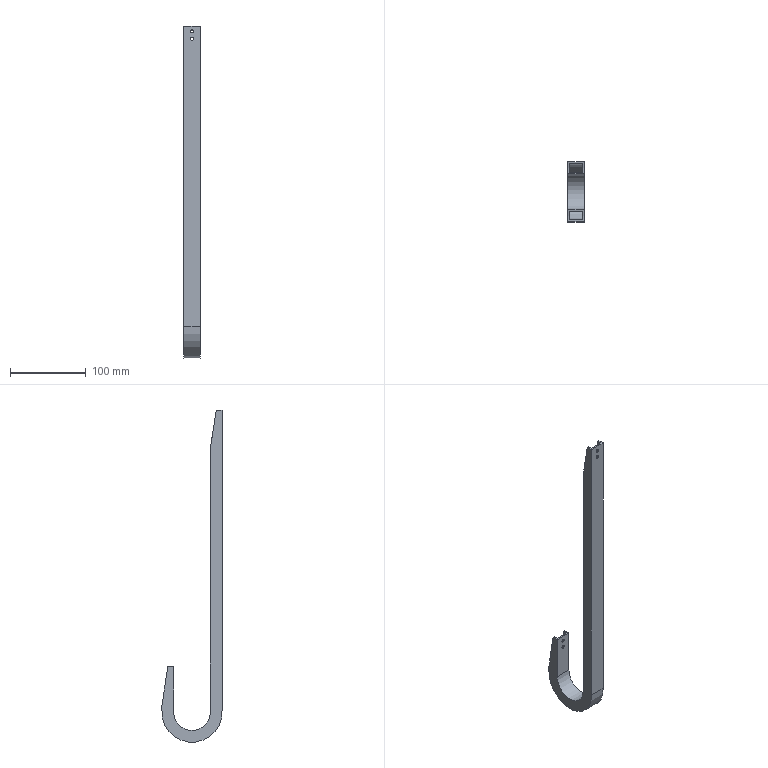Part | STEP file | ASND-0110-Body 1-7 | 1 solid | 30 faces | box 22 x 79.611 x 439.805 mm | volume 70298 mm3 | plane 16 | cylinder 14 | commonest cylinder face diameters 4 x8 75.611 x3 48.5 x1 52.5 x1 79.611 x1